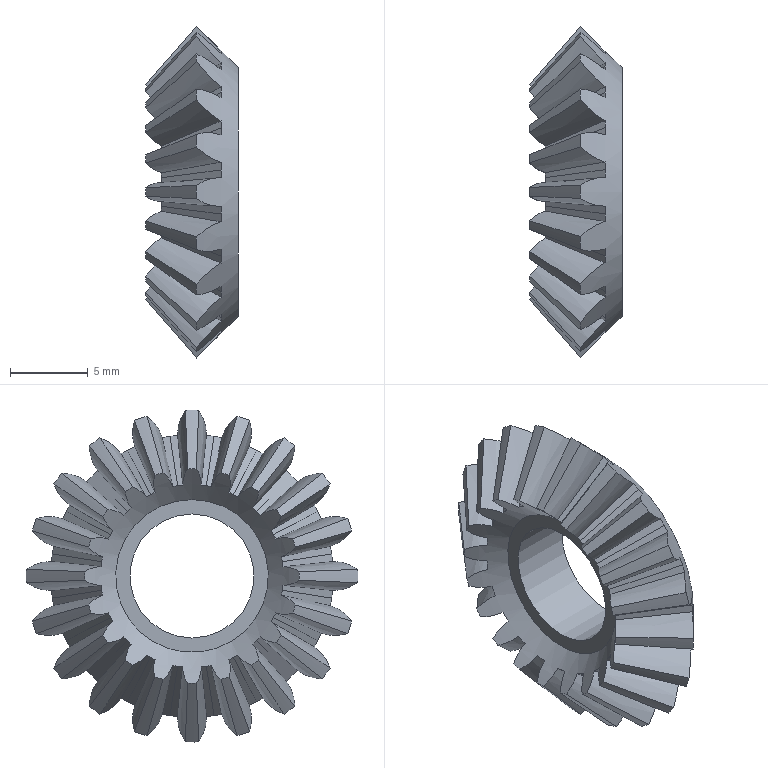Part | NX | features EXTRACT_BODY 20, TRIM BODY 20, Instance Feature 19, DATUM_CSYS 2, EXTEND_SHEET 1, Pattern Feature 1, SKETCH 1, SKIN 1, SWP104 1 | 1 solid | 105 faces | box 5.993 x 21.414 x 21.414 mm | volume 898.737 mm3 | plane 42 | spline 40 | cone 22 | cylinder 1 | commonest cylinder face diameters 8 x1